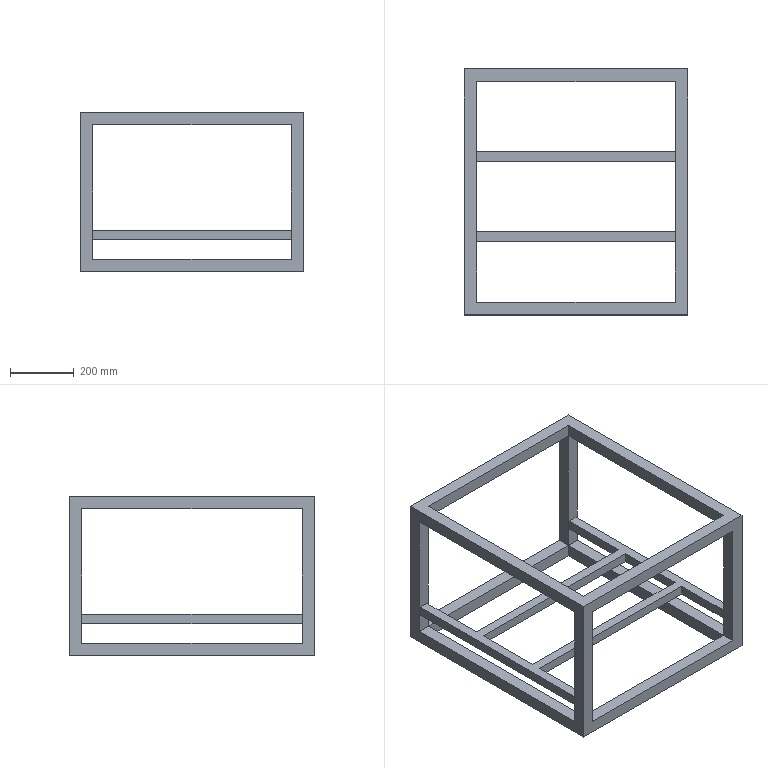Part | SolidWorks | features BaseBody 1 | 1 solid | 44 faces | box 700 x 770 x 500 mm | volume 13960000 mm3 | plane 44
STEP:
#1=CARTESIAN_POINT('',(-350.,-385.,-500.));
#2=VERTEX_POINT('',#1);
#3=CARTESIAN_POINT('',(350.,-385.,-500.));
#4=VERTEX_POINT('',#3);
#5=CARTESIAN_POINT('',(0.,-385.,-500.));
#6=DIRECTION('',(1.,0.,0.));
#7=VECTOR('',#6,1000.);
#8=LINE('',#5,#7);
#9=EDGE_CURVE('',#2,#4,#8,.T.);
#10=ORIENTED_EDGE('',*,*,#9,.F.);
#11=CARTESIAN_POINT('',(-350.,385.,-500.));
#12=VERTEX_POINT('',#11);
#13=CARTESIAN_POINT('',(-350.,0.,-500.));
#14=DIRECTION('',(0.,-1.,0.));
#15=VECTOR('',#14,1000.);
#16=LINE('',#13,#15);
#17=EDGE_CURVE('',#12,#2,#16,.T.);
#18=ORIENTED_EDGE('',*,*,#17,.F.);
#19=CARTESIAN_POINT('',(350.,385.,-500.));
#20=VERTEX_POINT('',#19);
#21=CARTESIAN_POINT('',(0.,385.,-500.));
#22=DIRECTION('',(-1.,0.,0.));
#23=VECTOR('',#22,1000.);
#24=LINE('',#21,#23);
#25=EDGE_CURVE('',#20,#12,#24,.T.);
#26=ORIENTED_EDGE('',*,*,#25,.F.);
#27=CARTESIAN_POINT('',(350.,0.,-500.));
#28=DIRECTION('',(0.,1.,0.));
#29=VECTOR('',#28,1000.);
#30=LINE('',#27,#29);
#31=EDGE_CURVE('',#4,#20,#30,.T.);
#32=ORIENTED_EDGE('',*,*,#31,.F.);
#33=EDGE_LOOP('',(#10,#18,#26,#32));
#34=FACE_OUTER_BOUND('',#33,.T.);
#35=CARTESIAN_POINT('',(310.,345.,-500.));
#36=VERTEX_POINT('',#35);
#37=CARTESIAN_POINT('',(310.,-345.,-500.));
#38=VERTEX_POINT('',#37);
#39=CARTESIAN_POINT('',(310.,0.,-500.));
#40=DIRECTION('',(0.,-1.,0.));
#41=VECTOR('',#40,1000.);
#42=LINE('',#39,#41);
#43=EDGE_CURVE('',#36,#38,#42,.T.);
#44=ORIENTED_EDGE('',*,*,#43,.F.);
#45=CARTESIAN_POINT('',(-310.,345.,-500.));
#46=VERTEX_POINT('',#45);
#47=CARTESIAN_POINT('',(0.,345.,-500.));
#48=DIRECTION('',(1.,0.,0.));
#49=VECTOR('',#48,1000.);
#50=LINE('',#47,#49);
#51=EDGE_CURVE('',#46,#36,#50,.T.);
#52=ORIENTED_EDGE('',*,*,#51,.F.);
#53=CARTESIAN_POINT('',(-310.,-345.,-500.));
#54=VERTEX_POINT('',#53);
#55=CARTESIAN_POINT('',(-310.,0.,-500.));
#56=DIRECTION('',(0.,1.,0.));
#57=VECTOR('',#56,1000.);
#58=LINE('',#55,#57);
#59=EDGE_CURVE('',#54,#46,#58,.T.);
#60=ORIENTED_EDGE('',*,*,#59,.F.);
#61=CARTESIAN_POINT('',(0.,-345.,-500.));
#62=DIRECTION('',(-1.,0.,0.));
#63=VECTOR('',#62,1000.);
#64=LINE('',#61,#63);
#65=EDGE_CURVE('',#38,#54,#64,.T.);
#66=ORIENTED_EDGE('',*,*,#65,.F.);
#67=EDGE_LOOP('',(#44,#52,#60,#66));
#68=FACE_BOUND('',#67,.T.);
#69=CARTESIAN_POINT('',(0.,0.,-500.));
#70=DIRECTION('',(0.,0.,1.));
#71=DIRECTION('',(1.,0.,0.));
#72=AXIS2_PLACEMENT_3D('',#69,#70,#71);
#73=PLANE('',#72);
#74=ADVANCED_FACE('',(#34,#68),#73,.F.);
#75=ORIENTED_EDGE('',*,*,#31,.T.);
#76=CARTESIAN_POINT('',(350.,385.,0.));
#77=VERTEX_POINT('',#76);
#78=CARTESIAN_POINT('',(350.,385.,-500.));
#79=DIRECTION('',(0.,0.,1.));
#80=VECTOR('',#79,1000.);
#81=LINE('',#78,#80);
#82=EDGE_CURVE('',#20,#77,#81,.T.);
#83=ORIENTED_EDGE('',*,*,#82,.T.);
#84=CARTESIAN_POINT('',(350.,-385.,0.));
#85=VERTEX_POINT('',#84);
#86=CARTESIAN_POINT('',(350.,385.,0.));
#87=DIRECTION('',(0.,-1.,0.));
#88=VECTOR('',#87,1000.);
#89=LINE('',#86,#88);
#90=EDGE_CURVE('',#77,#85,#89,.T.);
#91=ORIENTED_EDGE('',*,*,#90,.T.);
#92=CARTESIAN_POINT('',(350.,-385.,-500.));
#93=DIRECTION('',(0.,0.,-1.));
#94=VECTOR('',#93,1000.);
#95=LINE('',#92,#94);
#96=EDGE_CURVE('',#85,#4,#95,.T.);
#97=ORIENTED_EDGE('',*,*,#96,.T.);
#98=EDGE_LOOP('',(#75,#83,#91,#97));
#99=FACE_OUTER_BOUND('',#98,.T.);
#100=CARTESIAN_POINT('',(350.,-345.,-40.));
#101=VERTEX_POINT('',#100);
#102=CARTESIAN_POINT('',(350.,345.,-40.));
#103=VERTEX_POINT('',#102);
#104=CARTESIAN_POINT('',(350.,385.,-40.));
#105=DIRECTION('',(0.,1.,0.));
#106=VECTOR('',#105,1000.);
#107=LINE('',#104,#106);
#108=EDGE_CURVE('',#101,#103,#107,.T.);
#109=ORIENTED_EDGE('',*,*,#108,.T.);
#110=CARTESIAN_POINT('',(350.,345.,-460.));
#111=VERTEX_POINT('',#110);
#112=CARTESIAN_POINT('',(350.,345.,-500.));
#113=DIRECTION('',(0.,0.,-1.));
#114=VECTOR('',#113,1000.);
#115=LINE('',#112,#114);
#116=EDGE_CURVE('',#103,#111,#115,.T.);
#117=ORIENTED_EDGE('',*,*,#116,.T.);
#118=CARTESIAN_POINT('',(350.,-345.,-460.));
#119=VERTEX_POINT('',#118);
#120=CARTESIAN_POINT('',(350.,385.,-460.));
#121=DIRECTION('',(0.,-1.,0.));
#122=VECTOR('',#121,1000.);
#123=LINE('',#120,#122);
#124=EDGE_CURVE('',#111,#119,#123,.T.);
#125=ORIENTED_EDGE('',*,*,#124,.T.);
#126=CARTESIAN_POINT('',(350.,-345.,-500.));
#127=DIRECTION('',(0.,0.,1.));
#128=VECTOR('',#127,1000.);
#129=LINE('',#126,#128);
#130=EDGE_CURVE('',#119,#101,#129,.T.);
#131=ORIENTED_EDGE('',*,*,#130,.T.);
#132=EDGE_LOOP('',(#109,#117,#125,#131));
#133=FACE_BOUND('',#132,.T.);
#134=CARTESIAN_POINT('',(350.,385.,-500.));
#135=DIRECTION('',(1.,0.,0.));
#136=DIRECTION('',(0.,1.,0.));
#137=AXIS2_PLACEMENT_3D('',#134,#135,#136);
#138=PLANE('',#137);
#139=ADVANCED_FACE('',(#99,#133),#138,.T.);
#140=ORIENTED_EDGE('',*,*,#9,.T.);
#141=ORIENTED_EDGE('',*,*,#96,.F.);
#142=CARTESIAN_POINT('',(-350.,-385.,0.));
#143=VERTEX_POINT('',#142);
#144=CARTESIAN_POINT('',(-350.,-385.,0.));
#145=DIRECTION('',(-1.,0.,0.));
#146=VECTOR('',#145,1000.);
#147=LINE('',#144,#146);
#148=EDGE_CURVE('',#85,#143,#147,.T.);
#149=ORIENTED_EDGE('',*,*,#148,.T.);
#150=CARTESIAN_POINT('',(-350.,-385.,-500.));
#151=DIRECTION('',(0.,0.,-1.));
#152=VECTOR('',#151,1000.);
#153=LINE('',#150,#152);
#154=EDGE_CURVE('',#143,#2,#153,.T.);
#155=ORIENTED_EDGE('',*,*,#154,.T.);
#156=EDGE_LOOP('',(#140,#141,#149,#155));
#157=FACE_OUTER_BOUND('',#156,.T.);
#158=CARTESIAN_POINT('',(-310.,-385.,-460.));
#159=VERTEX_POINT('',#158);
#160=CARTESIAN_POINT('',(-310.,-385.,-40.));
#161=VERTEX_POINT('',#160);
#162=CARTESIAN_POINT('',(-310.,-385.,-500.));
#163=DIRECTION('',(0.,0.,1.));
#164=VECTOR('',#163,1000.);
#165=LINE('',#162,#164);
#166=EDGE_CURVE('',#159,#161,#165,.T.);
#167=ORIENTED_EDGE('',*,*,#166,.T.);
#168=CARTESIAN_POINT('',(310.,-385.,-40.));
#169=VERTEX_POINT('',#168);
#170=CARTESIAN_POINT('',(-350.,-385.,-40.));
#171=DIRECTION('',(1.,0.,0.));
#172=VECTOR('',#171,1000.);
#173=LINE('',#170,#172);
#174=EDGE_CURVE('',#161,#169,#173,.T.);
#175=ORIENTED_EDGE('',*,*,#174,.T.);
#176=CARTESIAN_POINT('',(310.,-385.,-460.));
#177=VERTEX_POINT('',#176);
#178=CARTESIAN_POINT('',(310.,-385.,-500.));
#179=DIRECTION('',(0.,0.,-1.));
#180=VECTOR('',#179,1000.);
#181=LINE('',#178,#180);
#182=EDGE_CURVE('',#169,#177,#181,.T.);
#183=ORIENTED_EDGE('',*,*,#182,.T.);
#184=CARTESIAN_POINT('',(-350.,-385.,-460.));
#185=DIRECTION('',(-1.,0.,0.));
#186=VECTOR('',#185,1000.);
#187=LINE('',#184,#186);
#188=EDGE_CURVE('',#177,#159,#187,.T.);
#189=ORIENTED_EDGE('',*,*,#188,.T.);
#190=EDGE_LOOP('',(#167,#175,#183,#189));
#191=FACE_BOUND('',#190,.T.);
#192=CARTESIAN_POINT('',(-350.,-385.,-500.));
#193=DIRECTION('',(0.,-1.,0.));
#194=DIRECTION('',(0.,0.,-1.));
#195=AXIS2_PLACEMENT_3D('',#192,#193,#194);
#196=PLANE('',#195);
#197=ADVANCED_FACE('',(#157,#191),#196,.T.);
#198=ORIENTED_EDGE('',*,*,#17,.T.);
#199=ORIENTED_EDGE('',*,*,#154,.F.);
#200=CARTESIAN_POINT('',(-350.,385.,0.));
#201=VERTEX_POINT('',#200);
#202=CARTESIAN_POINT('',(-350.,385.,0.));
#203=DIRECTION('',(0.,1.,0.));
#204=VECTOR('',#203,1000.);
#205=LINE('',#202,#204);
#206=EDGE_CURVE('',#143,#201,#205,.T.);
#207=ORIENTED_EDGE('',*,*,#206,.T.);
#208=CARTESIAN_POINT('',(-350.,385.,-500.));
#209=DIRECTION('',(0.,0.,-1.));
#210=VECTOR('',#209,1000.);
#211=LINE('',#208,#210);
#212=EDGE_CURVE('',#201,#12,#211,.T.);
#213=ORIENTED_EDGE('',*,*,#212,.T.);
#214=EDGE_LOOP('',(#198,#199,#207,#213));
#215=FACE_OUTER_BOUND('',#214,.T.);
#216=CARTESIAN_POINT('',(-350.,345.,-40.));
#217=VERTEX_POINT('',#216);
#218=CARTESIAN_POINT('',(-350.,-345.,-40.));
#219=VERTEX_POINT('',#218);
#220=CARTESIAN_POINT('',(-350.,385.,-40.));
#221=DIRECTION('',(0.,-1.,0.));
#222=VECTOR('',#221,1000.);
#223=LINE('',#220,#222);
#224=EDGE_CURVE('',#217,#219,#223,.T.);
#225=ORIENTED_EDGE('',*,*,#224,.T.);
#226=CARTESIAN_POINT('',(-350.,-345.,-460.));
#227=VERTEX_POINT('',#226);
#228=CARTESIAN_POINT('',(-350.,-345.,-500.));
#229=DIRECTION('',(0.,0.,-1.));
#230=VECTOR('',#229,1000.);
#231=LINE('',#228,#230);
#232=EDGE_CURVE('',#219,#227,#231,.T.);
#233=ORIENTED_EDGE('',*,*,#232,.T.);
#234=CARTESIAN_POINT('',(-350.,345.,-460.));
#235=VERTEX_POINT('',#234);
#236=CARTESIAN_POINT('',(-350.,385.,-460.));
#237=DIRECTION('',(0.,1.,0.));
#238=VECTOR('',#237,1000.);
#239=LINE('',#236,#238);
#240=EDGE_CURVE('',#227,#235,#239,.T.);
#241=ORIENTED_EDGE('',*,*,#240,.T.);
#242=CARTESIAN_POINT('',(-350.,345.,-500.));
#243=DIRECTION('',(0.,0.,1.));
#244=VECTOR('',#243,1000.);
#245=LINE('',#242,#244);
#246=EDGE_CURVE('',#235,#217,#245,.T.);
#247=ORIENTED_EDGE('',*,*,#246,.T.);
#248=EDGE_LOOP('',(#225,#233,#241,#247));
#249=FACE_BOUND('',#248,.T.);
#250=CARTESIAN_POINT('',(-350.,385.,-500.));
#251=DIRECTION('',(-1.,0.,0.));
#252=DIRECTION('',(0.,-1.,0.));
#253=AXIS2_PLACEMENT_3D('',#250,#251,#252);
#254=PLANE('',#253);
#255=ADVANCED_FACE('',(#215,#249),#254,.T.);
#256=ORIENTED_EDGE('',*,*,#25,.T.);
#257=ORIENTED_EDGE('',*,*,#212,.F.);
#258=CARTESIAN_POINT('',(-350.,385.,0.));
#259=DIRECTION('',(1.,0.,0.));
#260=VECTOR('',#259,1000.);
#261=LINE('',#258,#260);
#262=EDGE_CURVE('',#201,#77,#261,.T.);
#263=ORIENTED_EDGE('',*,*,#262,.T.);
#264=ORIENTED_EDGE('',*,*,#82,.F.);
#265=EDGE_LOOP('',(#256,#257,#263,#264));
#266=FACE_OUTER_BOUND('',#265,.T.);
#267=CARTESIAN_POINT('',(-310.,385.,-40.));
#268=VERTEX_POINT('',#267);
#269=CARTESIAN_POINT('',(-310.,385.,-460.));
#270=VERTEX_POINT('',#269);
#271=CARTESIAN_POINT('',(-310.,385.,-500.));
#272=DIRECTION('',(0.,0.,-1.));
#273=VECTOR('',#272,1000.);
#274=LINE('',#271,#273);
#275=EDGE_CURVE('',#268,#270,#274,.T.);
#276=ORIENTED_EDGE('',*,*,#275,.T.);
#277=CARTESIAN_POINT('',(310.,385.,-460.));
#278=VERTEX_POINT('',#277);
#279=CARTESIAN_POINT('',(-350.,385.,-460.));
#280=DIRECTION('',(1.,0.,0.));
#281=VECTOR('',#280,1000.);
#282=LINE('',#279,#281);
#283=EDGE_CURVE('',#270,#278,#282,.T.);
#284=ORIENTED_EDGE('',*,*,#283,.T.);
#285=CARTESIAN_POINT('',(310.,385.,-40.));
#286=VERTEX_POINT('',#285);
#287=CARTESIAN_POINT('',(310.,385.,-500.));
#288=DIRECTION('',(0.,0.,1.));
#289=VECTOR('',#288,1000.);
#290=LINE('',#287,#289);
#291=EDGE_CURVE('',#278,#286,#290,.T.);
#292=ORIENTED_EDGE('',*,*,#291,.T.);
#293=CARTESIAN_POINT('',(-350.,385.,-40.));
#294=DIRECTION('',(-1.,0.,0.));
#295=VECTOR('',#294,1000.);
#296=LINE('',#293,#295);
#297=EDGE_CURVE('',#286,#268,#296,.T.);
#298=ORIENTED_EDGE('',*,*,#297,.T.);
#299=EDGE_LOOP('',(#276,#284,#292,#298));
#300=FACE_BOUND('',#299,.T.);
#301=CARTESIAN_POINT('',(-350.,385.,-500.));
#302=DIRECTION('',(0.,1.,0.));
#303=DIRECTION('',(0.,0.,1.));
#304=AXIS2_PLACEMENT_3D('',#301,#302,#303);
#305=PLANE('',#304);
#306=ADVANCED_FACE('',(#266,#300),#305,.T.);
#307=CARTESIAN_POINT('',(310.,-345.,-460.));
#308=VERTEX_POINT('',#307);
#309=CARTESIAN_POINT('',(-310.,-345.,-460.));
#310=VERTEX_POINT('',#309);
#311=CARTESIAN_POINT('',(-310.,-345.,-460.));
#312=DIRECTION('',(-1.,0.,0.));
#313=VECTOR('',#312,1000.);
#314=LINE('',#311,#313);
#315=EDGE_CURVE('',#308,#310,#314,.T.);
#316=ORIENTED_EDGE('',*,*,#315,.F.);
#317=CARTESIAN_POINT('',(310.,-345.,-500.));
#318=DIRECTION('',(0.,0.,1.));
#319=VECTOR('',#318,1000.);
#320=LINE('',#317,#319);
#321=EDGE_CURVE('',#38,#308,#320,.T.);
#322=ORIENTED_EDGE('',*,*,#321,.F.);
#323=ORIENTED_EDGE('',*,*,#65,.T.);
#324=CARTESIAN_POINT('',(-310.,-345.,-500.));
#325=DIRECTION('',(0.,0.,-1.));
#326=VECTOR('',#325,1000.);
#327=LINE('',#324,#326);
#328=EDGE_CURVE('',#310,#54,#327,.T.);
#329=ORIENTED_EDGE('',*,*,#328,.F.);
#330=EDGE_LOOP('',(#316,#322,#323,#329));
#331=FACE_OUTER_BOUND('',#330,.T.);
#332=CARTESIAN_POINT('',(-310.,-345.,-500.));
#333=DIRECTION('',(0.,-1.,0.));
#334=DIRECTION('',(0.,0.,-1.));
#335=AXIS2_PLACEMENT_3D('',#332,#333,#334);
#336=PLANE('',#335);
#337=ADVANCED_FACE('',(#331),#336,.F.);
#338=CARTESIAN_POINT('',(310.,345.,-460.));
#339=VERTEX_POINT('',#338);
#340=CARTESIAN_POINT('',(310.,345.,-460.));
#341=DIRECTION('',(0.,-1.,0.));
#342=VECTOR('',#341,1000.);
#343=LINE('',#340,#342);
#344=EDGE_CURVE('',#339,#308,#343,.T.);
#345=ORIENTED_EDGE('',*,*,#344,.F.);
#346=CARTESIAN_POINT('',(310.,345.,-500.));
#347=DIRECTION('',(0.,0.,1.));
#348=VECTOR('',#347,1000.);
#349=LINE('',#346,#348);
#350=EDGE_CURVE('',#36,#339,#349,.T.);
#351=ORIENTED_EDGE('',*,*,#350,.F.);
#352=ORIENTED_EDGE('',*,*,#43,.T.);
#353=ORIENTED_EDGE('',*,*,#321,.T.);
#354=EDGE_LOOP('',(#345,#351,#352,#353));
#355=FACE_OUTER_BOUND('',#354,.T.);
#356=CARTESIAN_POINT('',(310.,345.,-500.));
#357=DIRECTION('',(1.,0.,0.));
#358=DIRECTION('',(0.,1.,0.));
#359=AXIS2_PLACEMENT_3D('',#356,#357,#358);
#360=PLANE('',#359);
#361=ADVANCED_FACE('',(#355),#360,.F.);
#362=CARTESIAN_POINT('',(-310.,345.,-460.));
#363=VERTEX_POINT('',#362);
#364=CARTESIAN_POINT('',(-310.,345.,-460.));
#365=DIRECTION('',(1.,0.,0.));
#366=VECTOR('',#365,1000.);
#367=LINE('',#364,#366);
#368=EDGE_CURVE('',#363,#339,#367,.T.);
#369=ORIENTED_EDGE('',*,*,#368,.F.);
#370=CARTESIAN_POINT('',(-310.,345.,-500.));
#371=DIRECTION('',(0.,0.,1.));
#372=VECTOR('',#371,1000.);
#373=LINE('',#370,#372);
#374=EDGE_CURVE('',#46,#363,#373,.T.);
#375=ORIENTED_EDGE('',*,*,#374,.F.);
#376=ORIENTED_EDGE('',*,*,#51,.T.);
#377=ORIENTED_EDGE('',*,*,#350,.T.);
#378=EDGE_LOOP('',(#369,#375,#376,#377));
#379=FACE_OUTER_BOUND('',#378,.T.);
#380=CARTESIAN_POINT('',(-310.,345.,-500.));
#381=DIRECTION('',(0.,1.,0.));
#382=DIRECTION('',(0.,0.,1.));
#383=AXIS2_PLACEMENT_3D('',#380,#381,#382);
#384=PLANE('',#383);
#385=ADVANCED_FACE('',(#379),#384,.F.);
#386=CARTESIAN_POINT('',(-310.,345.,-460.));
#387=DIRECTION('',(0.,1.,0.));
#388=VECTOR('',#387,1000.);
#389=LINE('',#386,#388);
#390=EDGE_CURVE('',#310,#363,#389,.T.);
#391=ORIENTED_EDGE('',*,*,#390,.F.);
#392=ORIENTED_EDGE('',*,*,#328,.T.);
#393=ORIENTED_EDGE('',*,*,#59,.T.);
#394=ORIENTED_EDGE('',*,*,#374,.T.);
#395=EDGE_LOOP('',(#391,#392,#393,#394));
#396=FACE_OUTER_BOUND('',#395,.T.);
#397=CARTESIAN_POINT('',(-310.,345.,-500.));
#398=DIRECTION('',(-1.,0.,0.));
#399=DIRECTION('',(0.,-1.,0.));
#400=AXIS2_PLACEMENT_3D('',#397,#398,#399);
#401=PLANE('',#400);
#402=ADVANCED_FACE('',(#396),#401,.F.);
#403=ORIENTED_EDGE('',*,*,#206,.F.);
#404=ORIENTED_EDGE('',*,*,#148,.F.);
#405=ORIENTED_EDGE('',*,*,#90,.F.);
#406=ORIENTED_EDGE('',*,*,#262,.F.);
#407=EDGE_LOOP('',(#403,#404,#405,#406));
#408=FACE_OUTER_BOUND('',#407,.T.);
#409=CARTESIAN_POINT('',(-310.,-345.,0.));
#410=VERTEX_POINT('',#409);
#411=CARTESIAN_POINT('',(-310.,345.,0.));
#412=VERTEX_POINT('',#411);
#413=CARTESIAN_POINT('',(-310.,0.,0.));
#414=DIRECTION('',(0.,1.,0.));
#415=VECTOR('',#414,1000.);
#416=LINE('',#413,#415);
#417=EDGE_CURVE('',#410,#412,#416,.T.);
#418=ORIENTED_EDGE('',*,*,#417,.T.);
#419=CARTESIAN_POINT('',(310.,345.,0.));
#420=VERTEX_POINT('',#419);
#421=CARTESIAN_POINT('',(0.,345.,0.));
#422=DIRECTION('',(1.,0.,0.));
#423=VECTOR('',#422,1000.);
#424=LINE('',#421,#423);
#425=EDGE_CURVE('',#412,#420,#424,.T.);
#426=ORIENTED_EDGE('',*,*,#425,.T.);
#427=CARTESIAN_POINT('',(310.,-345.,0.));
#428=VERTEX_POINT('',#427);
#429=CARTESIAN_POINT('',(310.,0.,0.));
#430=DIRECTION('',(0.,-1.,0.));
#431=VECTOR('',#430,1000.);
#432=LINE('',#429,#431);
#433=EDGE_CURVE('',#420,#428,#432,.T.);
#434=ORIENTED_EDGE('',*,*,#433,.T.);
#435=CARTESIAN_POINT('',(0.,-345.,0.));
#436=DIRECTION('',(-1.,0.,0.));
#437=VECTOR('',#436,1000.);
#438=LINE('',#435,#437);
#439=EDGE_CURVE('',#428,#410,#438,.T.);
#440=ORIENTED_EDGE('',*,*,#439,.T.);
#441=EDGE_LOOP('',(#418,#426,#434,#440));
#442=FACE_BOUND('',#441,.T.);
#443=CARTESIAN_POINT('',(0.,0.,0.));
#444=DIRECTION('',(0.,0.,1.));
#445=DIRECTION('',(1.,0.,0.));
#446=AXIS2_PLACEMENT_3D('',#443,#444,#445);
#447=PLANE('',#446);
#448=ADVANCED_FACE('',(#408,#442),#447,.T.);
#449=CARTESIAN_POINT('',(345.,345.,-370.));
#450=VERTEX_POINT('',#449);
#451=CARTESIAN_POINT('',(315.,345.,-370.));
#452=VERTEX_POINT('',#451);
#453=CARTESIAN_POINT('',(-350.,345.,-370.));
#454=DIRECTION('',(-1.,0.,0.));
#455=VECTOR('',#454,1000.);
#456=LINE('',#453,#455);
#457=EDGE_CURVE('',#450,#452,#456,.T.);
#458=ORIENTED_EDGE('',*,*,#457,.F.);
#459=CARTESIAN_POINT('',(345.,345.,-400.));
#460=VERTEX_POINT('',#459);
#461=CARTESIAN_POINT('',(345.,345.,-40.));
#462=DIRECTION('',(0.,0.,1.));
#463=VECTOR('',#462,1000.);
#464=LINE('',#461,#463);
#465=EDGE_CURVE('',#460,#450,#464,.T.);
#466=ORIENTED_EDGE('',*,*,#465,.F.);
#467=CARTESIAN_POINT('',(315.,345.,-400.));
#468=VERTEX_POINT('',#467);
#469=CARTESIAN_POINT('',(-350.,345.,-400.));
#470=DIRECTION('',(1.,0.,0.));
#471=VECTOR('',#470,1000.);
#472=LINE('',#469,#471);
#473=EDGE_CURVE('',#468,#460,#472,.T.);
#474=ORIENTED_EDGE('',*,*,#473,.F.);
#475=CARTESIAN_POINT('',(315.,345.,-40.));
#476=DIRECTION('',(0.,0.,-1.));
#477=VECTOR('',#476,1000.);
#478=LINE('',#475,#477);
#479=EDGE_CURVE('',#452,#468,#478,.T.);
#480=ORIENTED_EDGE('',*,*,#479,.F.);
#481=EDGE_LOOP('',(#458,#466,#474,#480));
#482=FACE_BOUND('',#481,.T.);
#483=ORIENTED_EDGE('',*,*,#116,.F.);
#484=CARTESIAN_POINT('',(310.,345.,-40.));
#485=VERTEX_POINT('',#484);
#486=CARTESIAN_POINT('',(-350.,345.,-40.));
#487=DIRECTION('',(1.,0.,0.));
#488=VECTOR('',#487,1000.);
#489=LINE('',#486,#488);
#490=EDGE_CURVE('',#485,#103,#489,.T.);
#491=ORIENTED_EDGE('',*,*,#490,.F.);
#492=CARTESIAN_POINT('',(310.,345.,-40.));
#493=DIRECTION('',(0.,0.,1.));
#494=VECTOR('',#493,1000.);
#495=LINE('',#492,#494);
#496=EDGE_CURVE('',#339,#485,#495,.T.);
#497=ORIENTED_EDGE('',*,*,#496,.F.);
#498=CARTESIAN_POINT('',(-350.,345.,-460.));
#499=DIRECTION('',(-1.,0.,0.));
#500=VECTOR('',#499,1000.);
#501=LINE('',#498,#500);
#502=EDGE_CURVE('',#111,#339,#501,.T.);
#503=ORIENTED_EDGE('',*,*,#502,.F.);
#504=EDGE_LOOP('',(#483,#491,#497,#503));
#505=FACE_OUTER_BOUND('',#504,.T.);
#506=CARTESIAN_POINT('',(-350.,345.,-40.));
#507=DIRECTION('',(0.,1.,0.));
#508=DIRECTION('',(-1.,0.,0.));
#509=AXIS2_PLACEMENT_3D('',#506,#507,#508);
#510=PLANE('',#509);
#511=ADVANCED_FACE('',(#482,#505),#510,.F.);
#512=ORIENTED_EDGE('',*,*,#108,.F.);
#513=CARTESIAN_POINT('',(310.,-345.,-40.));
#514=VERTEX_POINT('',#513);
#515=CARTESIAN_POINT('',(-350.,-345.,-40.));
#516=DIRECTION('',(1.,0.,0.));
#517=VECTOR('',#516,1000.);
#518=LINE('',#515,#517);
#519=EDGE_CURVE('',#514,#101,#518,.T.);
#520=ORIENTED_EDGE('',*,*,#519,.F.);
#521=CARTESIAN_POINT('',(310.,345.,-40.));
#522=DIRECTION('',(0.,-1.,0.));
#523=VECTOR('',#522,1000.);
#524=LINE('',#521,#523);
#525=EDGE_CURVE('',#485,#514,#524,.T.);
#526=ORIENTED_EDGE('',*,*,#525,.F.);
#527=ORIENTED_EDGE('',*,*,#490,.T.);
#528=EDGE_LOOP('',(#512,#520,#526,#527));
#529=FACE_OUTER_BOUND('',#528,.T.);
#530=CARTESIAN_POINT('',(-350.,345.,-40.));
#531=DIRECTION('',(0.,0.,1.));
#532=DIRECTION('',(0.,-1.,0.));
#533=AXIS2_PLACEMENT_3D('',#530,#531,#532);
#534=PLANE('',#533);
#535=ADVANCED_FACE('',(#529),#534,.F.);
#536=CARTESIAN_POINT('',(345.,-345.,-400.));
#537=VERTEX_POINT('',#536);
#538=CARTESIAN_POINT('',(315.,-345.,-400.));
#539=VERTEX_POINT('',#538);
#540=CARTESIAN_POINT('',(-350.,-345.,-400.));
#541=DIRECTION('',(-1.,0.,0.));
#542=VECTOR('',#541,1000.);
#543=LINE('',#540,#542);
#544=EDGE_CURVE('',#537,#539,#543,.T.);
#545=ORIENTED_EDGE('',*,*,#544,.F.);
#546=CARTESIAN_POINT('',(345.,-345.,-370.));
#547=VERTEX_POINT('',#546);
#548=CARTESIAN_POINT('',(345.,-345.,-40.));
#549=DIRECTION('',(0.,0.,-1.));
#550=VECTOR('',#549,1000.);
#551=LINE('',#548,#550);
#552=EDGE_CURVE('',#547,#537,#551,.T.);
#553=ORIENTED_EDGE('',*,*,#552,.F.);
#554=CARTESIAN_POINT('',(315.,-345.,-370.));
#555=VERTEX_POINT('',#554);
#556=CARTESIAN_POINT('',(-350.,-345.,-370.));
#557=DIRECTION('',(1.,0.,0.));
#558=VECTOR('',#557,1000.);
#559=LINE('',#556,#558);
#560=EDGE_CURVE('',#555,#547,#559,.T.);
#561=ORIENTED_EDGE('',*,*,#560,.F.);
#562=CARTESIAN_POINT('',(315.,-345.,-40.));
#563=DIRECTION('',(0.,0.,1.));
#564=VECTOR('',#563,1000.);
#565=LINE('',#562,#564);
#566=EDGE_CURVE('',#539,#555,#565,.T.);
#567=ORIENTED_EDGE('',*,*,#566,.F.);
#568=EDGE_LOOP('',(#545,#553,#561,#567));
#569=FACE_BOUND('',#568,.T.);
#570=ORIENTED_EDGE('',*,*,#130,.F.);
#571=CARTESIAN_POINT('',(-350.,-345.,-460.));
#572=DIRECTION('',(1.,0.,0.));
#573=VECTOR('',#572,1000.);
#574=LINE('',#571,#573);
#575=EDGE_CURVE('',#308,#119,#574,.T.);
#576=ORIENTED_EDGE('',*,*,#575,.F.);
#577=CARTESIAN_POINT('',(310.,-345.,-40.));
#578=DIRECTION('',(0.,0.,-1.));
#579=VECTOR('',#578,1000.);
#580=LINE('',#577,#579);
#581=EDGE_CURVE('',#514,#308,#580,.T.);
#582=ORIENTED_EDGE('',*,*,#581,.F.);
#583=ORIENTED_EDGE('',*,*,#519,.T.);
#584=EDGE_LOOP('',(#570,#576,#582,#583));
#585=FACE_OUTER_BOUND('',#584,.T.);
#586=CARTESIAN_POINT('',(-350.,-345.,-40.));
#587=DIRECTION('',(0.,-1.,0.));
#588=DIRECTION('',(1.,0.,0.));
#589=AXIS2_PLACEMENT_3D('',#586,#587,#588);
#590=PLANE('',#589);
#591=ADVANCED_FACE('',(#569,#585),#590,.F.);
#592=ORIENTED_EDGE('',*,*,#124,.F.);
#593=ORIENTED_EDGE('',*,*,#502,.T.);
#594=ORIENTED_EDGE('',*,*,#344,.T.);
#595=ORIENTED_EDGE('',*,*,#575,.T.);
#596=EDGE_LOOP('',(#592,#593,#594,#595));
#597=FACE_OUTER_BOUND('',#596,.T.);
#598=CARTESIAN_POINT('',(-350.,345.,-460.));
#599=DIRECTION('',(0.,0.,-1.));
#600=DIRECTION('',(0.,1.,0.));
#601=AXIS2_PLACEMENT_3D('',#598,#599,#600);
#602=PLANE('',#601);
#603=ADVANCED_FACE('',(#597),#602,.F.);
#604=ORIENTED_EDGE('',*,*,#174,.F.);
#605=CARTESIAN_POINT('',(-310.,-345.,-40.));
#606=VERTEX_POINT('',#605);
#607=CARTESIAN_POINT('',(-310.,-385.,-40.));
#608=DIRECTION('',(0.,-1.,0.));
#609=VECTOR('',#608,1000.);
#610=LINE('',#607,#609);
#611=EDGE_CURVE('',#606,#161,#610,.T.);
#612=ORIENTED_EDGE('',*,*,#611,.F.);
#613=CARTESIAN_POINT('',(-310.,-345.,-40.));
#614=DIRECTION('',(-1.,0.,0.));
#615=VECTOR('',#614,1000.);
#616=LINE('',#613,#615);
#617=EDGE_CURVE('',#514,#606,#616,.T.);
#618=ORIENTED_EDGE('',*,*,#617,.F.);
#619=CARTESIAN_POINT('',(310.,-385.,-40.));
#620=DIRECTION('',(0.,1.,0.));
#621=VECTOR('',#620,1000.);
#622=LINE('',#619,#621);
#623=EDGE_CURVE('',#169,#514,#622,.T.);
#624=ORIENTED_EDGE('',*,*,#623,.F.);
#625=EDGE_LOOP('',(#604,#612,#618,#624));
#626=FACE_OUTER_BOUND('',#625,.T.);
#627=CARTESIAN_POINT('',(-310.,-385.,-40.));
#628=DIRECTION('',(0.,0.,1.));
#629=DIRECTION('',(1.,0.,0.));
#630=AXIS2_PLACEMENT_3D('',#627,#628,#629);
#631=PLANE('',#630);
#632=ADVANCED_FACE('',(#626),#631,.F.);
#633=CARTESIAN_POINT('',(-310.,-345.,-500.));
#634=DIRECTION('',(0.,0.,-1.));
#635=VECTOR('',#634,1000.);
#636=LINE('',#633,#635);
#637=EDGE_CURVE('',#606,#310,#636,.T.);
#638=ORIENTED_EDGE('',*,*,#637,.F.);
#639=ORIENTED_EDGE('',*,*,#611,.T.);
#640=ORIENTED_EDGE('',*,*,#166,.F.);
#641=CARTESIAN_POINT('',(-310.,345.,-460.));
#642=DIRECTION('',(0.,-1.,0.));
#643=VECTOR('',#642,1000.);
#644=LINE('',#641,#643);
#645=EDGE_CURVE('',#310,#159,#644,.T.);
#646=ORIENTED_EDGE('',*,*,#645,.F.);
#647=EDGE_LOOP('',(#638,#639,#640,#646));
#648=FACE_OUTER_BOUND('',#647,.T.);
#649=CARTESIAN_POINT('',(-310.,345.,-500.));
#650=DIRECTION('',(-1.,0.,0.));
#651=DIRECTION('',(0.,-1.,0.));
#652=AXIS2_PLACEMENT_3D('',#649,#650,#651);
#653=PLANE('',#652);
#654=ADVANCED_FACE('',(#648),#653,.F.);
#655=ORIENTED_EDGE('',*,*,#188,.F.);
#656=CARTESIAN_POINT('',(310.,-385.,-460.));
#657=DIRECTION('',(0.,-1.,0.));
#658=VECTOR('',#657,1000.);
#659=LINE('',#656,#658);
#660=EDGE_CURVE('',#308,#177,#659,.T.);
#661=ORIENTED_EDGE('',*,*,#660,.F.);
#662=ORIENTED_EDGE('',*,*,#315,.T.);
#663=ORIENTED_EDGE('',*,*,#645,.T.);
#664=EDGE_LOOP('',(#655,#661,#662,#663));
#665=FACE_OUTER_BOUND('',#664,.T.);
#666=CARTESIAN_POINT('',(-310.,-385.,-460.));
#667=DIRECTION('',(0.,0.,-1.));
#668=DIRECTION('',(-1.,0.,0.));
#669=AXIS2_PLACEMENT_3D('',#666,#667,#668);
#670=PLANE('',#669);
#671=ADVANCED_FACE('',(#665),#670,.F.);
#672=ORIENTED_EDGE('',*,*,#581,.T.);
#673=ORIENTED_EDGE('',*,*,#660,.T.);
#674=ORIENTED_EDGE('',*,*,#182,.F.);
#675=ORIENTED_EDGE('',*,*,#623,.T.);
#676=EDGE_LOOP('',(#672,#673,#674,#675));
#677=FACE_OUTER_BOUND('',#676,.T.);
#678=CARTESIAN_POINT('',(310.,345.,-500.));
#679=DIRECTION('',(1.,0.,0.));
#680=DIRECTION('',(0.,1.,0.));
#681=AXIS2_PLACEMENT_3D('',#678,#679,#680);
#682=PLANE('',#681);
#683=ADVANCED_FACE('',(#677),#682,.F.);
#684=CARTESIAN_POINT('',(-345.,-345.,-370.));
#685=VERTEX_POINT('',#684);
#686=CARTESIAN_POINT('',(-315.,-345.,-370.));
#687=VERTEX_POINT('',#686);
#688=CARTESIAN_POINT('',(-350.,-345.,-370.));
#689=DIRECTION('',(1.,0.,0.));
#690=VECTOR('',#689,1000.);
#691=LINE('',#688,#690);
#692=EDGE_CURVE('',#685,#687,#691,.T.);
#693=ORIENTED_EDGE('',*,*,#692,.F.);
#694=CARTESIAN_POINT('',(-345.,-345.,-400.));
#695=VERTEX_POINT('',#694);
#696=CARTESIAN_POINT('',(-345.,-345.,-40.));
#697=DIRECTION('',(0.,0.,1.));
#698=VECTOR('',#697,1000.);
#699=LINE('',#696,#698);
#700=EDGE_CURVE('',#695,#685,#699,.T.);
#701=ORIENTED_EDGE('',*,*,#700,.F.);
#702=CARTESIAN_POINT('',(-315.,-345.,-400.));
#703=VERTEX_POINT('',#702);
#704=CARTESIAN_POINT('',(-350.,-345.,-400.));
#705=DIRECTION('',(-1.,0.,0.));
#706=VECTOR('',#705,1000.);
#707=LINE('',#704,#706);
#708=EDGE_CURVE('',#703,#695,#707,.T.);
#709=ORIENTED_EDGE('',*,*,#708,.F.);
#710=CARTESIAN_POINT('',(-315.,-345.,-40.));
#711=DIRECTION('',(0.,0.,-1.));
#712=VECTOR('',#711,1000.);
#713=LINE('',#710,#712);
#714=EDGE_CURVE('',#687,#703,#713,.T.);
#715=ORIENTED_EDGE('',*,*,#714,.F.);
#716=EDGE_LOOP('',(#693,#701,#709,#715));
#717=FACE_BOUND('',#716,.T.);
#718=ORIENTED_EDGE('',*,*,#232,.F.);
#719=CARTESIAN_POINT('',(-350.,-345.,-40.));
#720=DIRECTION('',(-1.,0.,0.));
#721=VECTOR('',#720,1000.);
#722=LINE('',#719,#721);
#723=EDGE_CURVE('',#606,#219,#722,.T.);
#724=ORIENTED_EDGE('',*,*,#723,.F.);
#725=ORIENTED_EDGE('',*,*,#637,.T.);
#726=CARTESIAN_POINT('',(-350.,-345.,-460.));
#727=DIRECTION('',(1.,0.,0.));
#728=VECTOR('',#727,1000.);
#729=LINE('',#726,#728);
#730=EDGE_CURVE('',#227,#310,#729,.T.);
#731=ORIENTED_EDGE('',*,*,#730,.F.);
#732=EDGE_LOOP('',(#718,#724,#725,#731));
#733=FACE_OUTER_BOUND('',#732,.T.);
#734=CARTESIAN_POINT('',(-350.,-345.,-40.));
#735=DIRECTION('',(0.,-1.,0.));
#736=DIRECTION('',(1.,0.,0.));
#737=AXIS2_PLACEMENT_3D('',#734,#735,#736);
#738=PLANE('',#737);
#739=ADVANCED_FACE('',(#717,#733),#738,.F.);
#740=ORIENTED_EDGE('',*,*,#224,.F.);
#741=CARTESIAN_POINT('',(-310.,345.,-40.));
#742=VERTEX_POINT('',#741);
#743=CARTESIAN_POINT('',(-350.,345.,-40.));
#744=DIRECTION('',(-1.,0.,0.));
#745=VECTOR('',#744,1000.);
#746=LINE('',#743,#745);
#747=EDGE_CURVE('',#742,#217,#746,.T.);
#748=ORIENTED_EDGE('',*,*,#747,.F.);
#749=CARTESIAN_POINT('',(-310.,345.,-40.));
#750=DIRECTION('',(0.,1.,0.));
#751=VECTOR('',#750,1000.);
#752=LINE('',#749,#751);
#753=EDGE_CURVE('',#606,#742,#752,.T.);
#754=ORIENTED_EDGE('',*,*,#753,.F.);
#755=ORIENTED_EDGE('',*,*,#723,.T.);
#756=EDGE_LOOP('',(#740,#748,#754,#755));
#757=FACE_OUTER_BOUND('',#756,.T.);
#758=CARTESIAN_POINT('',(-350.,345.,-40.));
#759=DIRECTION('',(0.,0.,1.));
#760=DIRECTION('',(0.,-1.,0.));
#761=AXIS2_PLACEMENT_3D('',#758,#759,#760);
#762=PLANE('',#761);
#763=ADVANCED_FACE('',(#757),#762,.F.);
#764=CARTESIAN_POINT('',(-345.,345.,-400.));
#765=VERTEX_POINT('',#764);
#766=CARTESIAN_POINT('',(-315.,345.,-400.));
#767=VERTEX_POINT('',#766);
#768=CARTESIAN_POINT('',(-350.,345.,-400.));
#769=DIRECTION('',(1.,0.,0.));
#770=VECTOR('',#769,1000.);
#771=LINE('',#768,#770);
#772=EDGE_CURVE('',#765,#767,#771,.T.);
#773=ORIENTED_EDGE('',*,*,#772,.F.);
#774=CARTESIAN_POINT('',(-345.,345.,-370.));
#775=VERTEX_POINT('',#774);
#776=CARTESIAN_POINT('',(-345.,345.,-40.));
#777=DIRECTION('',(0.,0.,-1.));
#778=VECTOR('',#777,1000.);
#779=LINE('',#776,#778);
#780=EDGE_CURVE('',#775,#765,#779,.T.);
#781=ORIENTED_EDGE('',*,*,#780,.F.);
#782=CARTESIAN_POINT('',(-315.,345.,-370.));
#783=VERTEX_POINT('',#782);
#784=CARTESIAN_POINT('',(-350.,345.,-370.));
#785=DIRECTION('',(-1.,0.,0.));
#786=VECTOR('',#785,1000.);
#787=LINE('',#784,#786);
#788=EDGE_CURVE('',#783,#775,#787,.T.);
#789=ORIENTED_EDGE('',*,*,#788,.F.);
#790=CARTESIAN_POINT('',(-315.,345.,-40.));
#791=DIRECTION('',(0.,0.,1.));
#792=VECTOR('',#791,1000.);
#793=LINE('',#790,#792);
#794=EDGE_CURVE('',#767,#783,#793,.T.);
#795=ORIENTED_EDGE('',*,*,#794,.F.);
#796=EDGE_LOOP('',(#773,#781,#789,#795));
#797=FACE_BOUND('',#796,.T.);
#798=ORIENTED_EDGE('',*,*,#246,.F.);
#799=CARTESIAN_POINT('',(-350.,345.,-460.));
#800=DIRECTION('',(-1.,0.,0.));
#801=VECTOR('',#800,1000.);
#802=LINE('',#799,#801);
#803=EDGE_CURVE('',#363,#235,#802,.T.);
#804=ORIENTED_EDGE('',*,*,#803,.F.);
#805=CARTESIAN_POINT('',(-310.,345.,-40.));
#806=DIRECTION('',(0.,0.,-1.));
#807=VECTOR('',#806,1000.);
#808=LINE('',#805,#807);
#809=EDGE_CURVE('',#742,#363,#808,.T.);
#810=ORIENTED_EDGE('',*,*,#809,.F.);
#811=ORIENTED_EDGE('',*,*,#747,.T.);
#812=EDGE_LOOP('',(#798,#804,#810,#811));
#813=FACE_OUTER_BOUND('',#812,.T.);
#814=CARTESIAN_POINT('',(-350.,345.,-40.));
#815=DIRECTION('',(0.,1.,0.));
#816=DIRECTION('',(-1.,0.,0.));
#817=AXIS2_PLACEMENT_3D('',#814,#815,#816);
#818=PLANE('',#817);
#819=ADVANCED_FACE('',(#797,#813),#818,.F.);
#820=ORIENTED_EDGE('',*,*,#240,.F.);
#821=ORIENTED_EDGE('',*,*,#730,.T.);
#822=ORIENTED_EDGE('',*,*,#390,.T.);
#823=ORIENTED_EDGE('',*,*,#803,.T.);
#824=EDGE_LOOP('',(#820,#821,#822,#823));
#825=FACE_OUTER_BOUND('',#824,.T.);
#826=CARTESIAN_POINT('',(-350.,345.,-460.));
#827=DIRECTION('',(0.,0.,-1.));
#828=DIRECTION('',(0.,1.,0.));
#829=AXIS2_PLACEMENT_3D('',#826,#827,#828);
#830=PLANE('',#829);
#831=ADVANCED_FACE('',(#825),#830,.F.);
#832=ORIENTED_EDGE('',*,*,#283,.F.);
#833=CARTESIAN_POINT('',(-310.,-385.,-460.));
#834=DIRECTION('',(0.,1.,0.));
#835=VECTOR('',#834,1000.);
#836=LINE('',#833,#835);
#837=EDGE_CURVE('',#363,#270,#836,.T.);
#838=ORIENTED_EDGE('',*,*,#837,.F.);
#839=ORIENTED_EDGE('',*,*,#368,.T.);
#840=CARTESIAN_POINT('',(310.,-385.,-460.));
#841=DIRECTION('',(0.,-1.,0.));
#842=VECTOR('',#841,1000.);
#843=LINE('',#840,#842);
#844=EDGE_CURVE('',#278,#339,#843,.T.);
#845=ORIENTED_EDGE('',*,*,#844,.F.);
#846=EDGE_LOOP('',(#832,#838,#839,#845));
#847=FACE_OUTER_BOUND('',#846,.T.);
#848=CARTESIAN_POINT('',(-310.,-385.,-460.));
#849=DIRECTION('',(0.,0.,-1.));
#850=DIRECTION('',(-1.,0.,0.));
#851=AXIS2_PLACEMENT_3D('',#848,#849,#850);
#852=PLANE('',#851);
#853=ADVANCED_FACE('',(#847),#852,.F.);
#854=ORIENTED_EDGE('',*,*,#809,.T.);
#855=ORIENTED_EDGE('',*,*,#837,.T.);
#856=ORIENTED_EDGE('',*,*,#275,.F.);
#857=CARTESIAN_POINT('',(-310.,345.,-40.));
#858=DIRECTION('',(0.,1.,0.));
#859=VECTOR('',#858,1000.);
#860=LINE('',#857,#859);
#861=EDGE_CURVE('',#742,#268,#860,.T.);
#862=ORIENTED_EDGE('',*,*,#861,.F.);
#863=EDGE_LOOP('',(#854,#855,#856,#862));
#864=FACE_OUTER_BOUND('',#863,.T.);
#865=CARTESIAN_POINT('',(-310.,345.,-500.));
#866=DIRECTION('',(-1.,0.,0.));
#867=DIRECTION('',(0.,-1.,0.));
#868=AXIS2_PLACEMENT_3D('',#865,#866,#867);
#869=PLANE('',#868);
#870=ADVANCED_FACE('',(#864),#869,.F.);
#871=ORIENTED_EDGE('',*,*,#297,.F.);
#872=CARTESIAN_POINT('',(310.,-385.,-40.));
#873=DIRECTION('',(0.,1.,0.));
#874=VECTOR('',#873,1000.);
#875=LINE('',#872,#874);
#876=EDGE_CURVE('',#485,#286,#875,.T.);
#877=ORIENTED_EDGE('',*,*,#876,.F.);
#878=CARTESIAN_POINT('',(-310.,345.,-40.));
#879=DIRECTION('',(1.,0.,0.));
#880=VECTOR('',#879,1000.);
#881=LINE('',#878,#880);
#882=EDGE_CURVE('',#742,#485,#881,.T.);
#883=ORIENTED_EDGE('',*,*,#882,.F.);
#884=ORIENTED_EDGE('',*,*,#861,.T.);
#885=EDGE_LOOP('',(#871,#877,#883,#884));
#886=FACE_OUTER_BOUND('',#885,.T.);
#887=CARTESIAN_POINT('',(-310.,-385.,-40.));
#888=DIRECTION('',(0.,0.,1.));
#889=DIRECTION('',(1.,0.,0.));
#890=AXIS2_PLACEMENT_3D('',#887,#888,#889);
#891=PLANE('',#890);
#892=ADVANCED_FACE('',(#886),#891,.F.);
#893=ORIENTED_EDGE('',*,*,#496,.T.);
#894=ORIENTED_EDGE('',*,*,#876,.T.);
#895=ORIENTED_EDGE('',*,*,#291,.F.);
#896=ORIENTED_EDGE('',*,*,#844,.T.);
#897=EDGE_LOOP('',(#893,#894,#895,#896));
#898=FACE_OUTER_BOUND('',#897,.T.);
#899=CARTESIAN_POINT('',(310.,345.,-500.));
#900=DIRECTION('',(1.,0.,0.));
#901=DIRECTION('',(0.,1.,0.));
#902=AXIS2_PLACEMENT_3D('',#899,#900,#901);
#903=PLANE('',#902);
#904=ADVANCED_FACE('',(#898),#903,.F.);
#905=ORIENTED_EDGE('',*,*,#882,.T.);
#906=CARTESIAN_POINT('',(310.,345.,-500.));
#907=DIRECTION('',(0.,0.,-1.));
#908=VECTOR('',#907,1000.);
#909=LINE('',#906,#908);
#910=EDGE_CURVE('',#420,#485,#909,.T.);
#911=ORIENTED_EDGE('',*,*,#910,.F.);
#912=ORIENTED_EDGE('',*,*,#425,.F.);
#913=CARTESIAN_POINT('',(-310.,345.,-500.));
#914=DIRECTION('',(0.,0.,1.));
#915=VECTOR('',#914,1000.);
#916=LINE('',#913,#915);
#917=EDGE_CURVE('',#742,#412,#916,.T.);
#918=ORIENTED_EDGE('',*,*,#917,.F.);
#919=EDGE_LOOP('',(#905,#911,#912,#918));
#920=FACE_OUTER_BOUND('',#919,.T.);
#921=CARTESIAN_POINT('',(-310.,345.,-500.));
#922=DIRECTION('',(0.,1.,0.));
#923=DIRECTION('',(0.,0.,1.));
#924=AXIS2_PLACEMENT_3D('',#921,#922,#923);
#925=PLANE('',#924);
#926=ADVANCED_FACE('',(#920),#925,.F.);
#927=ORIENTED_EDGE('',*,*,#753,.T.);
#928=ORIENTED_EDGE('',*,*,#917,.T.);
#929=ORIENTED_EDGE('',*,*,#417,.F.);
#930=CARTESIAN_POINT('',(-310.,-345.,-500.));
#931=DIRECTION('',(0.,0.,1.));
#932=VECTOR('',#931,1000.);
#933=LINE('',#930,#932);
#934=EDGE_CURVE('',#606,#410,#933,.T.);
#935=ORIENTED_EDGE('',*,*,#934,.F.);
#936=EDGE_LOOP('',(#927,#928,#929,#935));
#937=FACE_OUTER_BOUND('',#936,.T.);
#938=CARTESIAN_POINT('',(-310.,345.,-500.));
#939=DIRECTION('',(-1.,0.,0.));
#940=DIRECTION('',(0.,-1.,0.));
#941=AXIS2_PLACEMENT_3D('',#938,#939,#940);
#942=PLANE('',#941);
#943=ADVANCED_FACE('',(#937),#942,.F.);
#944=ORIENTED_EDGE('',*,*,#617,.T.);
#945=ORIENTED_EDGE('',*,*,#934,.T.);
#946=ORIENTED_EDGE('',*,*,#439,.F.);
#947=CARTESIAN_POINT('',(310.,-345.,-500.));
#948=DIRECTION('',(0.,0.,1.));
#949=VECTOR('',#948,1000.);
#950=LINE('',#947,#949);
#951=EDGE_CURVE('',#514,#428,#950,.T.);
#952=ORIENTED_EDGE('',*,*,#951,.F.);
#953=EDGE_LOOP('',(#944,#945,#946,#952));
#954=FACE_OUTER_BOUND('',#953,.T.);
#955=CARTESIAN_POINT('',(-310.,-345.,-500.));
#956=DIRECTION('',(0.,-1.,0.));
#957=DIRECTION('',(0.,0.,-1.));
#958=AXIS2_PLACEMENT_3D('',#955,#956,#957);
#959=PLANE('',#958);
#960=ADVANCED_FACE('',(#954),#959,.F.);
#961=ORIENTED_EDGE('',*,*,#525,.T.);
#962=ORIENTED_EDGE('',*,*,#951,.T.);
#963=ORIENTED_EDGE('',*,*,#433,.F.);
#964=ORIENTED_EDGE('',*,*,#910,.T.);
#965=EDGE_LOOP('',(#961,#962,#963,#964));
#966=FACE_OUTER_BOUND('',#965,.T.);
#967=CARTESIAN_POINT('',(310.,345.,-500.));
#968=DIRECTION('',(1.,0.,0.));
#969=DIRECTION('',(0.,1.,0.));
#970=AXIS2_PLACEMENT_3D('',#967,#968,#969);
#971=PLANE('',#970);
#972=ADVANCED_FACE('',(#966),#971,.F.);
#973=CARTESIAN_POINT('',(315.,126.5,-370.));
#974=VERTEX_POINT('',#973);
#975=CARTESIAN_POINT('',(315.,387.426,-370.));
#976=DIRECTION('',(0.,-1.,0.));
#977=VECTOR('',#976,1000.);
#978=LINE('',#975,#977);
#979=EDGE_CURVE('',#452,#974,#978,.T.);
#980=ORIENTED_EDGE('',*,*,#979,.F.);
#981=ORIENTED_EDGE('',*,*,#479,.T.);
#982=CARTESIAN_POINT('',(315.,126.5,-400.));
#983=VERTEX_POINT('',#982);
#984=CARTESIAN_POINT('',(315.,387.426,-400.));
#985=DIRECTION('',(0.,1.,0.));
#986=VECTOR('',#985,1000.);
#987=LINE('',#984,#986);
#988=EDGE_CURVE('',#983,#468,#987,.T.);
#989=ORIENTED_EDGE('',*,*,#988,.F.);
#990=CARTESIAN_POINT('',(315.,126.5,-370.));
#991=DIRECTION('',(0.,0.,-1.));
#992=VECTOR('',#991,1000.);
#993=LINE('',#990,#992);
#994=EDGE_CURVE('',#974,#983,#993,.T.);
#995=ORIENTED_EDGE('',*,*,#994,.F.);
#996=EDGE_LOOP('',(#980,#981,#989,#995));
#997=FACE_OUTER_BOUND('',#996,.T.);
#998=CARTESIAN_POINT('',(315.,387.426,-370.));
#999=DIRECTION('',(1.,0.,0.));
#1000=DIRECTION('',(0.,1.,0.));
#1001=AXIS2_PLACEMENT_3D('',#998,#999,#1000);
#1002=PLANE('',#1001);
#1003=ADVANCED_FACE('',(#997),#1002,.F.);
#1004=ORIENTED_EDGE('',*,*,#979,.T.);
#1005=CARTESIAN_POINT('',(-315.,126.5,-370.));
#1006=VERTEX_POINT('',#1005);
#1007=CARTESIAN_POINT('',(315.,126.5,-370.));
#1008=DIRECTION('',(1.,0.,0.));
#1009=VECTOR('',#1008,1000.);
#1010=LINE('',#1007,#1009);
#1011=EDGE_CURVE('',#1006,#974,#1010,.T.);
#1012=ORIENTED_EDGE('',*,*,#1011,.F.);
#1013=CARTESIAN_POINT('',(-315.,387.426,-370.));
#1014=DIRECTION('',(0.,-1.,0.));
#1015=VECTOR('',#1014,1000.);
#1016=LINE('',#1013,#1015);
#1017=EDGE_CURVE('',#783,#1006,#1016,.T.);
#1018=ORIENTED_EDGE('',*,*,#1017,.F.);
#1019=ORIENTED_EDGE('',*,*,#788,.T.);
#1020=CARTESIAN_POINT('',(-345.,387.426,-370.));
#1021=DIRECTION('',(0.,1.,0.));
#1022=VECTOR('',#1021,1000.);
#1023=LINE('',#1020,#1022);
#1024=EDGE_CURVE('',#685,#775,#1023,.T.);
#1025=ORIENTED_EDGE('',*,*,#1024,.F.);
#1026=ORIENTED_EDGE('',*,*,#692,.T.);
#1027=CARTESIAN_POINT('',(-315.,-153.5,-370.));
#1028=VERTEX_POINT('',#1027);
#1029=CARTESIAN_POINT('',(-315.,387.426,-370.));
#1030=DIRECTION('',(0.,-1.,0.));
#1031=VECTOR('',#1030,1000.);
#1032=LINE('',#1029,#1031);
#1033=EDGE_CURVE('',#1028,#687,#1032,.T.);
#1034=ORIENTED_EDGE('',*,*,#1033,.F.);
#1035=CARTESIAN_POINT('',(315.,-153.5,-370.));
#1036=VERTEX_POINT('',#1035);
#1037=CARTESIAN_POINT('',(315.,-153.5,-370.));
#1038=DIRECTION('',(-1.,0.,0.));
#1039=VECTOR('',#1038,1000.);
#1040=LINE('',#1037,#1039);
#1041=EDGE_CURVE('',#1036,#1028,#1040,.T.);
#1042=ORIENTED_EDGE('',*,*,#1041,.F.);
#1043=CARTESIAN_POINT('',(315.,387.426,-370.));
#1044=DIRECTION('',(0.,1.,0.));
#1045=VECTOR('',#1044,1000.);
#1046=LINE('',#1043,#1045);
#1047=EDGE_CURVE('',#555,#1036,#1046,.T.);
#1048=ORIENTED_EDGE('',*,*,#1047,.F.);
#1049=ORIENTED_EDGE('',*,*,#560,.T.);
#1050=CARTESIAN_POINT('',(345.,387.426,-370.));
#1051=DIRECTION('',(0.,-1.,0.));
#1052=VECTOR('',#1051,1000.);
#1053=LINE('',#1050,#1052);
#1054=EDGE_CURVE('',#450,#547,#1053,.T.);
#1055=ORIENTED_EDGE('',*,*,#1054,.F.);
#1056=ORIENTED_EDGE('',*,*,#457,.T.);
#1057=EDGE_LOOP('',(#1004,#1012,#1018,#1019,#1025,#1026,#1034,#1042,#1048,#1049,#1055,#1056));
#1058=FACE_OUTER_BOUND('',#1057,.T.);
#1059=CARTESIAN_POINT('',(315.,96.5,-370.));
#1060=VERTEX_POINT('',#1059);
#1061=CARTESIAN_POINT('',(-315.,96.5,-370.));
#1062=VERTEX_POINT('',#1061);
#1063=CARTESIAN_POINT('',(315.,96.5,-370.));
#1064=DIRECTION('',(-1.,0.,0.));
#1065=VECTOR('',#1064,1000.);
#1066=LINE('',#1063,#1065);
#1067=EDGE_CURVE('',#1060,#1062,#1066,.T.);
#1068=ORIENTED_EDGE('',*,*,#1067,.F.);
#1069=CARTESIAN_POINT('',(315.,-123.5,-370.));
#1070=VERTEX_POINT('',#1069);
#1071=CARTESIAN_POINT('',(315.,387.426,-370.));
#1072=DIRECTION('',(0.,1.,0.));
#1073=VECTOR('',#1072,1000.);
#1074=LINE('',#1071,#1073);
#1075=EDGE_CURVE('',#1070,#1060,#1074,.T.);
#1076=ORIENTED_EDGE('',*,*,#1075,.F.);
#1077=CARTESIAN_POINT('',(-315.,-123.5,-370.));
#1078=VERTEX_POINT('',#1077);
#1079=CARTESIAN_POINT('',(315.,-123.5,-370.));
#1080=DIRECTION('',(1.,0.,0.));
#1081=VECTOR('',#1080,1000.);
#1082=LINE('',#1079,#1081);
#1083=EDGE_CURVE('',#1078,#1070,#1082,.T.);
#1084=ORIENTED_EDGE('',*,*,#1083,.F.);
#1085=CARTESIAN_POINT('',(-315.,387.426,-370.));
#1086=DIRECTION('',(0.,-1.,0.));
#1087=VECTOR('',#1086,1000.);
#1088=LINE('',#1085,#1087);
#1089=EDGE_CURVE('',#1062,#1078,#1088,.T.);
#1090=ORIENTED_EDGE('',*,*,#1089,.F.);
#1091=EDGE_LOOP('',(#1068,#1076,#1084,#1090));
#1092=FACE_BOUND('',#1091,.T.);
#1093=CARTESIAN_POINT('',(315.,387.426,-370.));
#1094=DIRECTION('',(0.,0.,-1.));
#1095=DIRECTION('',(0.,1.,0.));
#1096=AXIS2_PLACEMENT_3D('',#1093,#1094,#1095);
#1097=PLANE('',#1096);
#1098=ADVANCED_FACE('',(#1058,#1092),#1097,.F.);
#1099=ORIENTED_EDGE('',*,*,#1054,.T.);
#1100=ORIENTED_EDGE('',*,*,#552,.T.);
#1101=CARTESIAN_POINT('',(345.,387.426,-400.));
#1102=DIRECTION('',(0.,-1.,0.));
#1103=VECTOR('',#1102,1000.);
#1104=LINE('',#1101,#1103);
#1105=EDGE_CURVE('',#460,#537,#1104,.T.);
#1106=ORIENTED_EDGE('',*,*,#1105,.F.);
#1107=ORIENTED_EDGE('',*,*,#465,.T.);
#1108=EDGE_LOOP('',(#1099,#1100,#1106,#1107));
#1109=FACE_OUTER_BOUND('',#1108,.T.);
#1110=CARTESIAN_POINT('',(345.,387.426,-370.));
#1111=DIRECTION('',(-1.,0.,0.));
#1112=DIRECTION('',(0.,-1.,0.));
#1113=AXIS2_PLACEMENT_3D('',#1110,#1111,#1112);
#1114=PLANE('',#1113);
#1115=ADVANCED_FACE('',(#1109),#1114,.F.);
#1116=CARTESIAN_POINT('',(-315.,-123.5,-400.));
#1117=VERTEX_POINT('',#1116);
#1118=CARTESIAN_POINT('',(-315.,96.5,-400.));
#1119=VERTEX_POINT('',#1118);
#1120=CARTESIAN_POINT('',(-315.,387.426,-400.));
#1121=DIRECTION('',(0.,1.,0.));
#1122=VECTOR('',#1121,1000.);
#1123=LINE('',#1120,#1122);
#1124=EDGE_CURVE('',#1117,#1119,#1123,.T.);
#1125=ORIENTED_EDGE('',*,*,#1124,.F.);
#1126=CARTESIAN_POINT('',(315.,-123.5,-400.));
#1127=VERTEX_POINT('',#1126);
#1128=CARTESIAN_POINT('',(315.,-123.5,-400.));
#1129=DIRECTION('',(-1.,0.,0.));
#1130=VECTOR('',#1129,1000.);
#1131=LINE('',#1128,#1130);
#1132=EDGE_CURVE('',#1127,#1117,#1131,.T.);
#1133=ORIENTED_EDGE('',*,*,#1132,.F.);
#1134=CARTESIAN_POINT('',(315.,96.5,-400.));
#1135=VERTEX_POINT('',#1134);
#1136=CARTESIAN_POINT('',(315.,387.426,-400.));
#1137=DIRECTION('',(0.,-1.,0.));
#1138=VECTOR('',#1137,1000.);
#1139=LINE('',#1136,#1138);
#1140=EDGE_CURVE('',#1135,#1127,#1139,.T.);
#1141=ORIENTED_EDGE('',*,*,#1140,.F.);
#1142=CARTESIAN_POINT('',(315.,96.5,-400.));
#1143=DIRECTION('',(1.,0.,0.));
#1144=VECTOR('',#1143,1000.);
#1145=LINE('',#1142,#1144);
#1146=EDGE_CURVE('',#1119,#1135,#1145,.T.);
#1147=ORIENTED_EDGE('',*,*,#1146,.F.);
#1148=EDGE_LOOP('',(#1125,#1133,#1141,#1147));
#1149=FACE_BOUND('',#1148,.T.);
#1150=CARTESIAN_POINT('',(-315.,126.5,-400.));
#1151=VERTEX_POINT('',#1150);
#1152=CARTESIAN_POINT('',(315.,126.5,-400.));
#1153=DIRECTION('',(-1.,0.,0.));
#1154=VECTOR('',#1153,1000.);
#1155=LINE('',#1152,#1154);
#1156=EDGE_CURVE('',#983,#1151,#1155,.T.);
#1157=ORIENTED_EDGE('',*,*,#1156,.F.);
#1158=ORIENTED_EDGE('',*,*,#988,.T.);
#1159=ORIENTED_EDGE('',*,*,#473,.T.);
#1160=ORIENTED_EDGE('',*,*,#1105,.T.);
#1161=ORIENTED_EDGE('',*,*,#544,.T.);
#1162=CARTESIAN_POINT('',(315.,-153.5,-400.));
#1163=VERTEX_POINT('',#1162);
#1164=CARTESIAN_POINT('',(315.,387.426,-400.));
#1165=DIRECTION('',(0.,-1.,0.));
#1166=VECTOR('',#1165,1000.);
#1167=LINE('',#1164,#1166);
#1168=EDGE_CURVE('',#1163,#539,#1167,.T.);
#1169=ORIENTED_EDGE('',*,*,#1168,.F.);
#1170=CARTESIAN_POINT('',(-315.,-153.5,-400.));
#1171=VERTEX_POINT('',#1170);
#1172=CARTESIAN_POINT('',(315.,-153.5,-400.));
#1173=DIRECTION('',(1.,0.,0.));
#1174=VECTOR('',#1173,1000.);
#1175=LINE('',#1172,#1174);
#1176=EDGE_CURVE('',#1171,#1163,#1175,.T.);
#1177=ORIENTED_EDGE('',*,*,#1176,.F.);
#1178=CARTESIAN_POINT('',(-315.,387.426,-400.));
#1179=DIRECTION('',(0.,1.,0.));
#1180=VECTOR('',#1179,1000.);
#1181=LINE('',#1178,#1180);
#1182=EDGE_CURVE('',#703,#1171,#1181,.T.);
#1183=ORIENTED_EDGE('',*,*,#1182,.F.);
#1184=ORIENTED_EDGE('',*,*,#708,.T.);
#1185=CARTESIAN_POINT('',(-345.,387.426,-400.));
#1186=DIRECTION('',(0.,-1.,0.));
#1187=VECTOR('',#1186,1000.);
#1188=LINE('',#1185,#1187);
#1189=EDGE_CURVE('',#765,#695,#1188,.T.);
#1190=ORIENTED_EDGE('',*,*,#1189,.F.);
#1191=ORIENTED_EDGE('',*,*,#772,.T.);
#1192=CARTESIAN_POINT('',(-315.,387.426,-400.));
#1193=DIRECTION('',(0.,1.,0.));
#1194=VECTOR('',#1193,1000.);
#1195=LINE('',#1192,#1194);
#1196=EDGE_CURVE('',#1151,#767,#1195,.T.);
#1197=ORIENTED_EDGE('',*,*,#1196,.F.);
#1198=EDGE_LOOP('',(#1157,#1158,#1159,#1160,#1161,#1169,#1177,#1183,#1184,#1190,#1191,#1197));
#1199=FACE_OUTER_BOUND('',#1198,.T.);
#1200=CARTESIAN_POINT('',(315.,387.426,-400.));
#1201=DIRECTION('',(0.,0.,1.));
#1202=DIRECTION('',(0.,-1.,0.));
#1203=AXIS2_PLACEMENT_3D('',#1200,#1201,#1202);
#1204=PLANE('',#1203);
#1205=ADVANCED_FACE('',(#1149,#1199),#1204,.F.);
#1206=ORIENTED_EDGE('',*,*,#1168,.T.);
#1207=ORIENTED_EDGE('',*,*,#566,.T.);
#1208=ORIENTED_EDGE('',*,*,#1047,.T.);
#1209=CARTESIAN_POINT('',(315.,-153.5,-370.));
#1210=DIRECTION('',(0.,0.,1.));
#1211=VECTOR('',#1210,1000.);
#1212=LINE('',#1209,#1211);
#1213=EDGE_CURVE('',#1163,#1036,#1212,.T.);
#1214=ORIENTED_EDGE('',*,*,#1213,.F.);
#1215=EDGE_LOOP('',(#1206,#1207,#1208,#1214));
#1216=FACE_OUTER_BOUND('',#1215,.T.);
#1217=CARTESIAN_POINT('',(315.,387.426,-370.));
#1218=DIRECTION('',(1.,0.,0.));
#1219=DIRECTION('',(0.,1.,0.));
#1220=AXIS2_PLACEMENT_3D('',#1217,#1218,#1219);
#1221=PLANE('',#1220);
#1222=ADVANCED_FACE('',(#1216),#1221,.F.);
#1223=ORIENTED_EDGE('',*,*,#1033,.T.);
#1224=ORIENTED_EDGE('',*,*,#714,.T.);
#1225=ORIENTED_EDGE('',*,*,#1182,.T.);
#1226=CARTESIAN_POINT('',(-315.,-153.5,-400.));
#1227=DIRECTION('',(0.,0.,-1.));
#1228=VECTOR('',#1227,1000.);
#1229=LINE('',#1226,#1228);
#1230=EDGE_CURVE('',#1028,#1171,#1229,.T.);
#1231=ORIENTED_EDGE('',*,*,#1230,.F.);
#1232=EDGE_LOOP('',(#1223,#1224,#1225,#1231));
#1233=FACE_OUTER_BOUND('',#1232,.T.);
#1234=CARTESIAN_POINT('',(-315.,387.426,-400.));
#1235=DIRECTION('',(-1.,0.,0.));
#1236=DIRECTION('',(0.,0.,1.));
#1237=AXIS2_PLACEMENT_3D('',#1234,#1235,#1236);
#1238=PLANE('',#1237);
#1239=ADVANCED_FACE('',(#1233),#1238,.F.);
#1240=ORIENTED_EDGE('',*,*,#1189,.T.);
#1241=ORIENTED_EDGE('',*,*,#700,.T.);
#1242=ORIENTED_EDGE('',*,*,#1024,.T.);
#1243=ORIENTED_EDGE('',*,*,#780,.T.);
#1244=EDGE_LOOP('',(#1240,#1241,#1242,#1243));
#1245=FACE_OUTER_BOUND('',#1244,.T.);
#1246=CARTESIAN_POINT('',(-345.,387.426,-400.));
#1247=DIRECTION('',(1.,0.,0.));
#1248=DIRECTION('',(0.,1.,0.));
#1249=AXIS2_PLACEMENT_3D('',#1246,#1247,#1248);
#1250=PLANE('',#1249);
#1251=ADVANCED_FACE('',(#1245),#1250,.F.);
#1252=ORIENTED_EDGE('',*,*,#1196,.T.);
#1253=ORIENTED_EDGE('',*,*,#794,.T.);
#1254=ORIENTED_EDGE('',*,*,#1017,.T.);
#1255=CARTESIAN_POINT('',(-315.,126.5,-400.));
#1256=DIRECTION('',(0.,0.,1.));
#1257=VECTOR('',#1256,1000.);
#1258=LINE('',#1255,#1257);
#1259=EDGE_CURVE('',#1151,#1006,#1258,.T.);
#1260=ORIENTED_EDGE('',*,*,#1259,.F.);
#1261=EDGE_LOOP('',(#1252,#1253,#1254,#1260));
#1262=FACE_OUTER_BOUND('',#1261,.T.);
#1263=CARTESIAN_POINT('',(-315.,387.426,-400.));
#1264=DIRECTION('',(-1.,0.,0.));
#1265=DIRECTION('',(0.,0.,1.));
#1266=AXIS2_PLACEMENT_3D('',#1263,#1264,#1265);
#1267=PLANE('',#1266);
#1268=ADVANCED_FACE('',(#1262),#1267,.F.);
#1269=ORIENTED_EDGE('',*,*,#1156,.T.);
#1270=ORIENTED_EDGE('',*,*,#1259,.T.);
#1271=ORIENTED_EDGE('',*,*,#1011,.T.);
#1272=ORIENTED_EDGE('',*,*,#994,.T.);
#1273=EDGE_LOOP('',(#1269,#1270,#1271,#1272));
#1274=FACE_OUTER_BOUND('',#1273,.T.);
#1275=CARTESIAN_POINT('',(357.426,126.5,-370.));
#1276=DIRECTION('',(0.,-1.,0.));
#1277=DIRECTION('',(1.,0.,0.));
#1278=AXIS2_PLACEMENT_3D('',#1275,#1276,#1277);
#1279=PLANE('',#1278);
#1280=ADVANCED_FACE('',(#1274),#1279,.F.);
#1281=ORIENTED_EDGE('',*,*,#1041,.T.);
#1282=ORIENTED_EDGE('',*,*,#1230,.T.);
#1283=ORIENTED_EDGE('',*,*,#1176,.T.);
#1284=ORIENTED_EDGE('',*,*,#1213,.T.);
#1285=EDGE_LOOP('',(#1281,#1282,#1283,#1284));
#1286=FACE_OUTER_BOUND('',#1285,.T.);
#1287=CARTESIAN_POINT('',(357.426,-153.5,-370.));
#1288=DIRECTION('',(0.,1.,0.));
#1289=DIRECTION('',(-1.,0.,0.));
#1290=AXIS2_PLACEMENT_3D('',#1287,#1288,#1289);
#1291=PLANE('',#1290);
#1292=ADVANCED_FACE('',(#1286),#1291,.F.);
#1293=ORIENTED_EDGE('',*,*,#1089,.T.);
#1294=CARTESIAN_POINT('',(-315.,-123.5,-400.));
#1295=DIRECTION('',(0.,0.,1.));
#1296=VECTOR('',#1295,1000.);
#1297=LINE('',#1294,#1296);
#1298=EDGE_CURVE('',#1117,#1078,#1297,.T.);
#1299=ORIENTED_EDGE('',*,*,#1298,.F.);
#1300=ORIENTED_EDGE('',*,*,#1124,.T.);
#1301=CARTESIAN_POINT('',(-315.,96.5,-400.));
#1302=DIRECTION('',(0.,0.,-1.));
#1303=VECTOR('',#1302,1000.);
#1304=LINE('',#1301,#1303);
#1305=EDGE_CURVE('',#1062,#1119,#1304,.T.);
#1306=ORIENTED_EDGE('',*,*,#1305,.F.);
#1307=EDGE_LOOP('',(#1293,#1299,#1300,#1306));
#1308=FACE_OUTER_BOUND('',#1307,.T.);
#1309=CARTESIAN_POINT('',(-315.,387.426,-400.));
#1310=DIRECTION('',(-1.,0.,0.));
#1311=DIRECTION('',(0.,0.,1.));
#1312=AXIS2_PLACEMENT_3D('',#1309,#1310,#1311);
#1313=PLANE('',#1312);
#1314=ADVANCED_FACE('',(#1308),#1313,.F.);
#1315=ORIENTED_EDGE('',*,*,#1067,.T.);
#1316=ORIENTED_EDGE('',*,*,#1305,.T.);
#1317=ORIENTED_EDGE('',*,*,#1146,.T.);
#1318=CARTESIAN_POINT('',(315.,96.5,-370.));
#1319=DIRECTION('',(0.,0.,-1.));
#1320=VECTOR('',#1319,1000.);
#1321=LINE('',#1318,#1320);
#1322=EDGE_CURVE('',#1060,#1135,#1321,.T.);
#1323=ORIENTED_EDGE('',*,*,#1322,.F.);
#1324=EDGE_LOOP('',(#1315,#1316,#1317,#1323));
#1325=FACE_OUTER_BOUND('',#1324,.T.);
#1326=CARTESIAN_POINT('',(357.426,96.5,-370.));
#1327=DIRECTION('',(0.,1.,0.));
#1328=DIRECTION('',(-1.,0.,0.));
#1329=AXIS2_PLACEMENT_3D('',#1326,#1327,#1328);
#1330=PLANE('',#1329);
#1331=ADVANCED_FACE('',(#1325),#1330,.F.);
#1332=ORIENTED_EDGE('',*,*,#1140,.T.);
#1333=CARTESIAN_POINT('',(315.,-123.5,-370.));
#1334=DIRECTION('',(0.,0.,-1.));
#1335=VECTOR('',#1334,1000.);
#1336=LINE('',#1333,#1335);
#1337=EDGE_CURVE('',#1070,#1127,#1336,.T.);
#1338=ORIENTED_EDGE('',*,*,#1337,.F.);
#1339=ORIENTED_EDGE('',*,*,#1075,.T.);
#1340=ORIENTED_EDGE('',*,*,#1322,.T.);
#1341=EDGE_LOOP('',(#1332,#1338,#1339,#1340));
#1342=FACE_OUTER_BOUND('',#1341,.T.);
#1343=CARTESIAN_POINT('',(315.,387.426,-370.));
#1344=DIRECTION('',(1.,0.,0.));
#1345=DIRECTION('',(0.,1.,0.));
#1346=AXIS2_PLACEMENT_3D('',#1343,#1344,#1345);
#1347=PLANE('',#1346);
#1348=ADVANCED_FACE('',(#1342),#1347,.F.);
#1349=ORIENTED_EDGE('',*,*,#1132,.T.);
#1350=ORIENTED_EDGE('',*,*,#1298,.T.);
#1351=ORIENTED_EDGE('',*,*,#1083,.T.);
#1352=ORIENTED_EDGE('',*,*,#1337,.T.);
#1353=EDGE_LOOP('',(#1349,#1350,#1351,#1352));
#1354=FACE_OUTER_BOUND('',#1353,.T.);
#1355=CARTESIAN_POINT('',(357.426,-123.5,-370.));
#1356=DIRECTION('',(0.,-1.,0.));
#1357=DIRECTION('',(1.,0.,0.));
#1358=AXIS2_PLACEMENT_3D('',#1355,#1356,#1357);
#1359=PLANE('',#1358);
#1360=ADVANCED_FACE('',(#1354),#1359,.F.);
#1361=CLOSED_SHELL('',(#74,#139,#197,#255,#306,#337,#361,#385,#402,#448,#511,#535,#591,#603,#632,#654,#671,#683,#739,#763,#819,#831,#853,#870,#892,#904,#926,#943,#960,#972,#1003,#1098,#1115,#1205,#1222,#1239,#1251,#1268,#1280,#1292,#1314,#1331,#1348,#1360));
#1362=MANIFOLD_SOLID_BREP('',#1361);
#1363=CARTESIAN_POINT('',(0.,0.,0.));
#1364=DIRECTION('',(0.,0.,1.));
#1365=DIRECTION('',(1.,0.,0.));
#1366=AXIS2_PLACEMENT_3D('',#1363,#1364,#1365);
#1367=(LENGTH_UNIT()NAMED_UNIT(*)SI_UNIT(.MILLI.,.METRE.));
#1368=UNCERTAINTY_MEASURE_WITH_UNIT(LENGTH_MEASURE(0.00001),#1367,'','');
#1369=(NAMED_UNIT(*)PLANE_ANGLE_UNIT()SI_UNIT($,.RADIAN.));
#1370=(NAMED_UNIT(*)SI_UNIT($,.STERADIAN.)SOLID_ANGLE_UNIT());
#1371=(GEOMETRIC_REPRESENTATION_CONTEXT(3)GLOBAL_UNCERTAINTY_ASSIGNED_CONTEXT((#1368))GLOBAL_UNIT_ASSIGNED_CONTEXT((#1367,#1369,#1370))REPRESENTATION_CONTEXT('',''));
#1372=ADVANCED_BREP_SHAPE_REPRESENTATION('',(#1362,#1366),#1371);